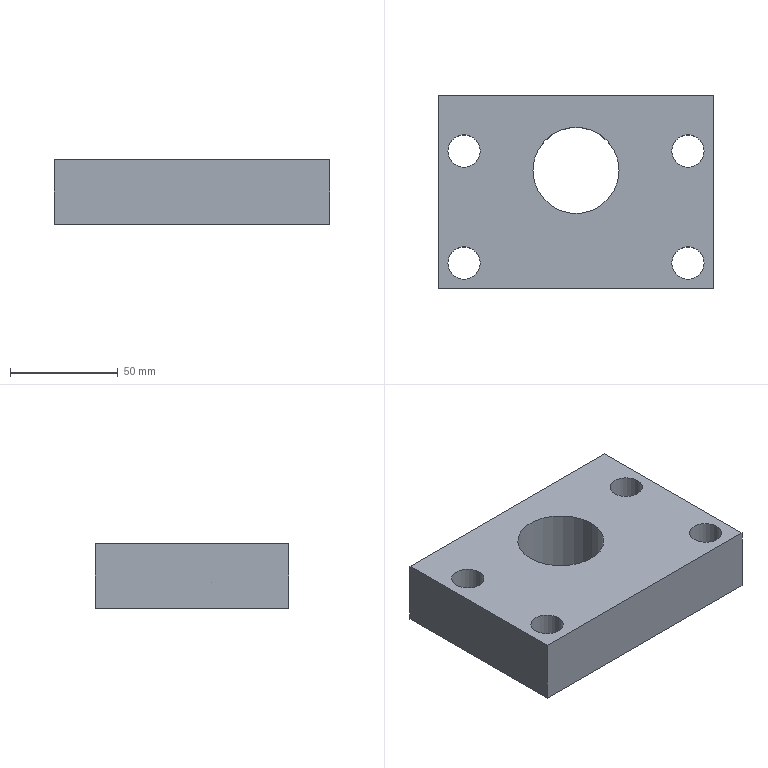Part | SolidWorks | features Extrusion 1, HoleWzd 1, ICE 1 | 1 solid | 16 faces | box 128 x 90 x 30 mm | volume 286695 mm3 | cylinder 10 | plane 6 | commonest cylinder face diameters 15 x8 40 x2
STEP:
#1=CARTESIAN_POINT('',(-59.5,19.,0.));
#2=VERTEX_POINT('',#1);
#3=CARTESIAN_POINT('',(-44.5,19.,0.));
#4=VERTEX_POINT('',#3);
#5=CARTESIAN_POINT('',(-52.,19.,0.));
#6=DIRECTION('',(0.,0.,1.));
#7=DIRECTION('',(1.,0.,0.));
#8=AXIS2_PLACEMENT_3D('',#5,#6,#7);
#9=CIRCLE('',#8,7.5);
#10=EDGE_CURVE('',#2,#4,#9,.T.);
#11=ORIENTED_EDGE('',*,*,#10,.F.);
#12=CARTESIAN_POINT('',(-59.5,19.,30.));
#13=VERTEX_POINT('',#12);
#14=CARTESIAN_POINT('',(-59.5,19.,30.));
#15=DIRECTION('',(0.,0.,1.));
#16=VECTOR('',#15,1000.);
#17=LINE('',#14,#16);
#18=EDGE_CURVE('',#2,#13,#17,.T.);
#19=ORIENTED_EDGE('',*,*,#18,.T.);
#20=CARTESIAN_POINT('',(-44.5,19.,30.));
#21=VERTEX_POINT('',#20);
#22=CARTESIAN_POINT('',(-52.,19.,30.));
#23=DIRECTION('',(0.,0.,1.));
#24=DIRECTION('',(1.,0.,0.));
#25=AXIS2_PLACEMENT_3D('',#22,#23,#24);
#26=CIRCLE('',#25,7.5);
#27=EDGE_CURVE('',#13,#21,#26,.T.);
#28=ORIENTED_EDGE('',*,*,#27,.T.);
#29=CARTESIAN_POINT('',(-44.5,19.,30.));
#30=DIRECTION('',(0.,0.,1.));
#31=VECTOR('',#30,1000.);
#32=LINE('',#29,#31);
#33=EDGE_CURVE('',#4,#21,#32,.T.);
#34=ORIENTED_EDGE('',*,*,#33,.F.);
#35=EDGE_LOOP('',(#11,#19,#28,#34));
#36=FACE_OUTER_BOUND('',#35,.T.);
#37=CARTESIAN_POINT('',(-52.,19.,30.));
#38=DIRECTION('',(0.,0.,1.));
#39=DIRECTION('',(1.,0.,0.));
#40=AXIS2_PLACEMENT_3D('',#37,#38,#39);
#41=CYLINDRICAL_SURFACE('',#40,7.5);
#42=ADVANCED_FACE('',(#36),#41,.F.);
#43=CARTESIAN_POINT('',(-59.5,-33.,0.));
#44=VERTEX_POINT('',#43);
#45=CARTESIAN_POINT('',(-44.5,-33.,0.));
#46=VERTEX_POINT('',#45);
#47=CARTESIAN_POINT('',(-52.,-33.,0.));
#48=DIRECTION('',(0.,0.,1.));
#49=DIRECTION('',(1.,0.,0.));
#50=AXIS2_PLACEMENT_3D('',#47,#48,#49);
#51=CIRCLE('',#50,7.5);
#52=EDGE_CURVE('',#44,#46,#51,.T.);
#53=ORIENTED_EDGE('',*,*,#52,.F.);
#54=CARTESIAN_POINT('',(-59.5,-33.,30.));
#55=VERTEX_POINT('',#54);
#56=CARTESIAN_POINT('',(-59.5,-33.,30.));
#57=DIRECTION('',(0.,0.,1.));
#58=VECTOR('',#57,1000.);
#59=LINE('',#56,#58);
#60=EDGE_CURVE('',#44,#55,#59,.T.);
#61=ORIENTED_EDGE('',*,*,#60,.T.);
#62=CARTESIAN_POINT('',(-44.5,-33.,30.));
#63=VERTEX_POINT('',#62);
#64=CARTESIAN_POINT('',(-52.,-33.,30.));
#65=DIRECTION('',(0.,0.,1.));
#66=DIRECTION('',(1.,0.,0.));
#67=AXIS2_PLACEMENT_3D('',#64,#65,#66);
#68=CIRCLE('',#67,7.5);
#69=EDGE_CURVE('',#55,#63,#68,.T.);
#70=ORIENTED_EDGE('',*,*,#69,.T.);
#71=CARTESIAN_POINT('',(-44.5,-33.,30.));
#72=DIRECTION('',(0.,0.,1.));
#73=VECTOR('',#72,1000.);
#74=LINE('',#71,#73);
#75=EDGE_CURVE('',#46,#63,#74,.T.);
#76=ORIENTED_EDGE('',*,*,#75,.F.);
#77=EDGE_LOOP('',(#53,#61,#70,#76));
#78=FACE_OUTER_BOUND('',#77,.T.);
#79=CARTESIAN_POINT('',(-52.,-33.,30.));
#80=DIRECTION('',(0.,0.,1.));
#81=DIRECTION('',(1.,0.,0.));
#82=AXIS2_PLACEMENT_3D('',#79,#80,#81);
#83=CYLINDRICAL_SURFACE('',#82,7.5);
#84=ADVANCED_FACE('',(#78),#83,.F.);
#85=CARTESIAN_POINT('',(44.5,-33.,0.));
#86=VERTEX_POINT('',#85);
#87=CARTESIAN_POINT('',(59.5,-33.,0.));
#88=VERTEX_POINT('',#87);
#89=CARTESIAN_POINT('',(52.,-33.,0.));
#90=DIRECTION('',(0.,0.,1.));
#91=DIRECTION('',(1.,0.,0.));
#92=AXIS2_PLACEMENT_3D('',#89,#90,#91);
#93=CIRCLE('',#92,7.5);
#94=EDGE_CURVE('',#86,#88,#93,.T.);
#95=ORIENTED_EDGE('',*,*,#94,.F.);
#96=CARTESIAN_POINT('',(44.5,-33.,30.));
#97=VERTEX_POINT('',#96);
#98=CARTESIAN_POINT('',(44.5,-33.,30.));
#99=DIRECTION('',(0.,0.,1.));
#100=VECTOR('',#99,1000.);
#101=LINE('',#98,#100);
#102=EDGE_CURVE('',#86,#97,#101,.T.);
#103=ORIENTED_EDGE('',*,*,#102,.T.);
#104=CARTESIAN_POINT('',(59.5,-33.,30.));
#105=VERTEX_POINT('',#104);
#106=CARTESIAN_POINT('',(52.,-33.,30.));
#107=DIRECTION('',(0.,0.,1.));
#108=DIRECTION('',(1.,0.,0.));
#109=AXIS2_PLACEMENT_3D('',#106,#107,#108);
#110=CIRCLE('',#109,7.5);
#111=EDGE_CURVE('',#97,#105,#110,.T.);
#112=ORIENTED_EDGE('',*,*,#111,.T.);
#113=CARTESIAN_POINT('',(59.5,-33.,30.));
#114=DIRECTION('',(0.,0.,1.));
#115=VECTOR('',#114,1000.);
#116=LINE('',#113,#115);
#117=EDGE_CURVE('',#88,#105,#116,.T.);
#118=ORIENTED_EDGE('',*,*,#117,.F.);
#119=EDGE_LOOP('',(#95,#103,#112,#118));
#120=FACE_OUTER_BOUND('',#119,.T.);
#121=CARTESIAN_POINT('',(52.,-33.,30.));
#122=DIRECTION('',(0.,0.,1.));
#123=DIRECTION('',(1.,0.,0.));
#124=AXIS2_PLACEMENT_3D('',#121,#122,#123);
#125=CYLINDRICAL_SURFACE('',#124,7.5);
#126=ADVANCED_FACE('',(#120),#125,.F.);
#127=CARTESIAN_POINT('',(44.5,19.,0.));
#128=VERTEX_POINT('',#127);
#129=CARTESIAN_POINT('',(59.5,19.,0.));
#130=VERTEX_POINT('',#129);
#131=CARTESIAN_POINT('',(52.,19.,0.));
#132=DIRECTION('',(0.,0.,1.));
#133=DIRECTION('',(1.,0.,0.));
#134=AXIS2_PLACEMENT_3D('',#131,#132,#133);
#135=CIRCLE('',#134,7.5);
#136=EDGE_CURVE('',#128,#130,#135,.T.);
#137=ORIENTED_EDGE('',*,*,#136,.F.);
#138=CARTESIAN_POINT('',(44.5,19.,30.));
#139=VERTEX_POINT('',#138);
#140=CARTESIAN_POINT('',(44.5,19.,30.));
#141=DIRECTION('',(0.,0.,1.));
#142=VECTOR('',#141,1000.);
#143=LINE('',#140,#142);
#144=EDGE_CURVE('',#128,#139,#143,.T.);
#145=ORIENTED_EDGE('',*,*,#144,.T.);
#146=CARTESIAN_POINT('',(59.5,19.,30.));
#147=VERTEX_POINT('',#146);
#148=CARTESIAN_POINT('',(52.,19.,30.));
#149=DIRECTION('',(0.,0.,1.));
#150=DIRECTION('',(1.,0.,0.));
#151=AXIS2_PLACEMENT_3D('',#148,#149,#150);
#152=CIRCLE('',#151,7.5);
#153=EDGE_CURVE('',#139,#147,#152,.T.);
#154=ORIENTED_EDGE('',*,*,#153,.T.);
#155=CARTESIAN_POINT('',(59.5,19.,30.));
#156=DIRECTION('',(0.,0.,1.));
#157=VECTOR('',#156,1000.);
#158=LINE('',#155,#157);
#159=EDGE_CURVE('',#130,#147,#158,.T.);
#160=ORIENTED_EDGE('',*,*,#159,.F.);
#161=EDGE_LOOP('',(#137,#145,#154,#160));
#162=FACE_OUTER_BOUND('',#161,.T.);
#163=CARTESIAN_POINT('',(52.,19.,30.));
#164=DIRECTION('',(0.,0.,1.));
#165=DIRECTION('',(1.,0.,0.));
#166=AXIS2_PLACEMENT_3D('',#163,#164,#165);
#167=CYLINDRICAL_SURFACE('',#166,7.5);
#168=ADVANCED_FACE('',(#162),#167,.F.);
#169=CARTESIAN_POINT('',(-20.,10.,0.));
#170=VERTEX_POINT('',#169);
#171=CARTESIAN_POINT('',(20.,10.,0.));
#172=VERTEX_POINT('',#171);
#173=CARTESIAN_POINT('',(0.,10.,0.));
#174=DIRECTION('',(0.,0.,1.));
#175=DIRECTION('',(1.,0.,0.));
#176=AXIS2_PLACEMENT_3D('',#173,#174,#175);
#177=CIRCLE('',#176,20.);
#178=EDGE_CURVE('',#170,#172,#177,.T.);
#179=ORIENTED_EDGE('',*,*,#178,.F.);
#180=CARTESIAN_POINT('',(-20.,10.,30.));
#181=VERTEX_POINT('',#180);
#182=CARTESIAN_POINT('',(-20.,10.,0.));
#183=DIRECTION('',(0.,0.,1.));
#184=VECTOR('',#183,1000.);
#185=LINE('',#182,#184);
#186=EDGE_CURVE('',#170,#181,#185,.T.);
#187=ORIENTED_EDGE('',*,*,#186,.T.);
#188=CARTESIAN_POINT('',(20.,10.,30.));
#189=VERTEX_POINT('',#188);
#190=CARTESIAN_POINT('',(0.,10.,30.));
#191=DIRECTION('',(0.,0.,1.));
#192=DIRECTION('',(1.,0.,0.));
#193=AXIS2_PLACEMENT_3D('',#190,#191,#192);
#194=CIRCLE('',#193,20.);
#195=EDGE_CURVE('',#181,#189,#194,.T.);
#196=ORIENTED_EDGE('',*,*,#195,.T.);
#197=CARTESIAN_POINT('',(20.,10.,0.));
#198=DIRECTION('',(0.,0.,1.));
#199=VECTOR('',#198,1000.);
#200=LINE('',#197,#199);
#201=EDGE_CURVE('',#172,#189,#200,.T.);
#202=ORIENTED_EDGE('',*,*,#201,.F.);
#203=EDGE_LOOP('',(#179,#187,#196,#202));
#204=FACE_OUTER_BOUND('',#203,.T.);
#205=CARTESIAN_POINT('',(0.,10.,0.));
#206=DIRECTION('',(0.,0.,1.));
#207=DIRECTION('',(1.,0.,0.));
#208=AXIS2_PLACEMENT_3D('',#205,#206,#207);
#209=CYLINDRICAL_SURFACE('',#208,20.);
#210=ADVANCED_FACE('',(#204),#209,.F.);
#211=CARTESIAN_POINT('',(-64.,45.,0.));
#212=VERTEX_POINT('',#211);
#213=CARTESIAN_POINT('',(-64.,-45.,0.));
#214=VERTEX_POINT('',#213);
#215=CARTESIAN_POINT('',(-64.,-45.,0.));
#216=DIRECTION('',(0.,-1.,0.));
#217=VECTOR('',#216,1000.);
#218=LINE('',#215,#217);
#219=EDGE_CURVE('',#212,#214,#218,.T.);
#220=ORIENTED_EDGE('',*,*,#219,.T.);
#221=CARTESIAN_POINT('',(-64.,-45.,30.));
#222=VERTEX_POINT('',#221);
#223=CARTESIAN_POINT('',(-64.,-45.,30.));
#224=DIRECTION('',(0.,0.,-1.));
#225=VECTOR('',#224,1000.);
#226=LINE('',#223,#225);
#227=EDGE_CURVE('',#222,#214,#226,.T.);
#228=ORIENTED_EDGE('',*,*,#227,.F.);
#229=CARTESIAN_POINT('',(-64.,45.,30.));
#230=VERTEX_POINT('',#229);
#231=CARTESIAN_POINT('',(-64.,-45.,30.));
#232=DIRECTION('',(0.,-1.,0.));
#233=VECTOR('',#232,1000.);
#234=LINE('',#231,#233);
#235=EDGE_CURVE('',#230,#222,#234,.T.);
#236=ORIENTED_EDGE('',*,*,#235,.F.);
#237=CARTESIAN_POINT('',(-64.,45.,30.));
#238=DIRECTION('',(0.,0.,-1.));
#239=VECTOR('',#238,1000.);
#240=LINE('',#237,#239);
#241=EDGE_CURVE('',#230,#212,#240,.T.);
#242=ORIENTED_EDGE('',*,*,#241,.T.);
#243=EDGE_LOOP('',(#220,#228,#236,#242));
#244=FACE_OUTER_BOUND('',#243,.T.);
#245=CARTESIAN_POINT('',(-64.,-45.,30.));
#246=DIRECTION('',(1.,0.,0.));
#247=DIRECTION('',(0.,0.,-1.));
#248=AXIS2_PLACEMENT_3D('',#245,#246,#247);
#249=PLANE('',#248);
#250=ADVANCED_FACE('',(#244),#249,.F.);
#251=CARTESIAN_POINT('',(64.,-45.,0.));
#252=VERTEX_POINT('',#251);
#253=CARTESIAN_POINT('',(64.,-45.,0.));
#254=DIRECTION('',(1.,0.,0.));
#255=VECTOR('',#254,1000.);
#256=LINE('',#253,#255);
#257=EDGE_CURVE('',#214,#252,#256,.T.);
#258=ORIENTED_EDGE('',*,*,#257,.T.);
#259=CARTESIAN_POINT('',(64.,-45.,30.));
#260=VERTEX_POINT('',#259);
#261=CARTESIAN_POINT('',(64.,-45.,30.));
#262=DIRECTION('',(0.,0.,-1.));
#263=VECTOR('',#262,1000.);
#264=LINE('',#261,#263);
#265=EDGE_CURVE('',#260,#252,#264,.T.);
#266=ORIENTED_EDGE('',*,*,#265,.F.);
#267=CARTESIAN_POINT('',(64.,-45.,30.));
#268=DIRECTION('',(1.,0.,0.));
#269=VECTOR('',#268,1000.);
#270=LINE('',#267,#269);
#271=EDGE_CURVE('',#222,#260,#270,.T.);
#272=ORIENTED_EDGE('',*,*,#271,.F.);
#273=ORIENTED_EDGE('',*,*,#227,.T.);
#274=EDGE_LOOP('',(#258,#266,#272,#273));
#275=FACE_OUTER_BOUND('',#274,.T.);
#276=CARTESIAN_POINT('',(64.,-45.,30.));
#277=DIRECTION('',(0.,1.,0.));
#278=DIRECTION('',(-1.,0.,0.));
#279=AXIS2_PLACEMENT_3D('',#276,#277,#278);
#280=PLANE('',#279);
#281=ADVANCED_FACE('',(#275),#280,.F.);
#282=CARTESIAN_POINT('',(64.,45.,0.));
#283=VERTEX_POINT('',#282);
#284=CARTESIAN_POINT('',(64.,-45.,0.));
#285=DIRECTION('',(0.,1.,0.));
#286=VECTOR('',#285,1000.);
#287=LINE('',#284,#286);
#288=EDGE_CURVE('',#252,#283,#287,.T.);
#289=ORIENTED_EDGE('',*,*,#288,.T.);
#290=CARTESIAN_POINT('',(64.,45.,30.));
#291=VERTEX_POINT('',#290);
#292=CARTESIAN_POINT('',(64.,45.,30.));
#293=DIRECTION('',(0.,0.,-1.));
#294=VECTOR('',#293,1000.);
#295=LINE('',#292,#294);
#296=EDGE_CURVE('',#291,#283,#295,.T.);
#297=ORIENTED_EDGE('',*,*,#296,.F.);
#298=CARTESIAN_POINT('',(64.,-45.,30.));
#299=DIRECTION('',(0.,1.,0.));
#300=VECTOR('',#299,1000.);
#301=LINE('',#298,#300);
#302=EDGE_CURVE('',#260,#291,#301,.T.);
#303=ORIENTED_EDGE('',*,*,#302,.F.);
#304=ORIENTED_EDGE('',*,*,#265,.T.);
#305=EDGE_LOOP('',(#289,#297,#303,#304));
#306=FACE_OUTER_BOUND('',#305,.T.);
#307=CARTESIAN_POINT('',(64.,-45.,30.));
#308=DIRECTION('',(-1.,0.,0.));
#309=DIRECTION('',(0.,0.,1.));
#310=AXIS2_PLACEMENT_3D('',#307,#308,#309);
#311=PLANE('',#310);
#312=ADVANCED_FACE('',(#306),#311,.F.);
#313=CARTESIAN_POINT('',(64.,45.,0.));
#314=DIRECTION('',(-1.,0.,0.));
#315=VECTOR('',#314,1000.);
#316=LINE('',#313,#315);
#317=EDGE_CURVE('',#283,#212,#316,.T.);
#318=ORIENTED_EDGE('',*,*,#317,.T.);
#319=ORIENTED_EDGE('',*,*,#241,.F.);
#320=CARTESIAN_POINT('',(64.,45.,30.));
#321=DIRECTION('',(-1.,0.,0.));
#322=VECTOR('',#321,1000.);
#323=LINE('',#320,#322);
#324=EDGE_CURVE('',#291,#230,#323,.T.);
#325=ORIENTED_EDGE('',*,*,#324,.F.);
#326=ORIENTED_EDGE('',*,*,#296,.T.);
#327=EDGE_LOOP('',(#318,#319,#325,#326));
#328=FACE_OUTER_BOUND('',#327,.T.);
#329=CARTESIAN_POINT('',(64.,45.,30.));
#330=DIRECTION('',(0.,-1.,0.));
#331=DIRECTION('',(1.,0.,0.));
#332=AXIS2_PLACEMENT_3D('',#329,#330,#331);
#333=PLANE('',#332);
#334=ADVANCED_FACE('',(#328),#333,.F.);
#335=CARTESIAN_POINT('',(-52.,19.,30.));
#336=DIRECTION('',(0.,0.,1.));
#337=DIRECTION('',(1.,0.,0.));
#338=AXIS2_PLACEMENT_3D('',#335,#336,#337);
#339=CIRCLE('',#338,7.5);
#340=EDGE_CURVE('',#21,#13,#339,.T.);
#341=ORIENTED_EDGE('',*,*,#340,.F.);
#342=ORIENTED_EDGE('',*,*,#27,.F.);
#343=EDGE_LOOP('',(#341,#342));
#344=FACE_BOUND('',#343,.T.);
#345=CARTESIAN_POINT('',(-52.,-33.,30.));
#346=DIRECTION('',(0.,0.,1.));
#347=DIRECTION('',(1.,0.,0.));
#348=AXIS2_PLACEMENT_3D('',#345,#346,#347);
#349=CIRCLE('',#348,7.5);
#350=EDGE_CURVE('',#63,#55,#349,.T.);
#351=ORIENTED_EDGE('',*,*,#350,.F.);
#352=ORIENTED_EDGE('',*,*,#69,.F.);
#353=EDGE_LOOP('',(#351,#352));
#354=FACE_BOUND('',#353,.T.);
#355=CARTESIAN_POINT('',(52.,-33.,30.));
#356=DIRECTION('',(0.,0.,1.));
#357=DIRECTION('',(1.,0.,0.));
#358=AXIS2_PLACEMENT_3D('',#355,#356,#357);
#359=CIRCLE('',#358,7.5);
#360=EDGE_CURVE('',#105,#97,#359,.T.);
#361=ORIENTED_EDGE('',*,*,#360,.F.);
#362=ORIENTED_EDGE('',*,*,#111,.F.);
#363=EDGE_LOOP('',(#361,#362));
#364=FACE_BOUND('',#363,.T.);
#365=CARTESIAN_POINT('',(52.,19.,30.));
#366=DIRECTION('',(0.,0.,1.));
#367=DIRECTION('',(1.,0.,0.));
#368=AXIS2_PLACEMENT_3D('',#365,#366,#367);
#369=CIRCLE('',#368,7.5);
#370=EDGE_CURVE('',#147,#139,#369,.T.);
#371=ORIENTED_EDGE('',*,*,#370,.F.);
#372=ORIENTED_EDGE('',*,*,#153,.F.);
#373=EDGE_LOOP('',(#371,#372));
#374=FACE_BOUND('',#373,.T.);
#375=CARTESIAN_POINT('',(0.,10.,30.));
#376=DIRECTION('',(0.,0.,1.));
#377=DIRECTION('',(1.,0.,0.));
#378=AXIS2_PLACEMENT_3D('',#375,#376,#377);
#379=CIRCLE('',#378,20.);
#380=EDGE_CURVE('',#189,#181,#379,.T.);
#381=ORIENTED_EDGE('',*,*,#380,.F.);
#382=ORIENTED_EDGE('',*,*,#195,.F.);
#383=EDGE_LOOP('',(#381,#382));
#384=FACE_BOUND('',#383,.T.);
#385=ORIENTED_EDGE('',*,*,#235,.T.);
#386=ORIENTED_EDGE('',*,*,#271,.T.);
#387=ORIENTED_EDGE('',*,*,#302,.T.);
#388=ORIENTED_EDGE('',*,*,#324,.T.);
#389=EDGE_LOOP('',(#385,#386,#387,#388));
#390=FACE_OUTER_BOUND('',#389,.T.);
#391=CARTESIAN_POINT('',(0.,0.,30.));
#392=DIRECTION('',(0.,0.,1.));
#393=DIRECTION('',(1.,0.,0.));
#394=AXIS2_PLACEMENT_3D('',#391,#392,#393);
#395=PLANE('',#394);
#396=ADVANCED_FACE('',(#344,#354,#364,#374,#384,#390),#395,.T.);
#397=CARTESIAN_POINT('',(-52.,19.,0.));
#398=DIRECTION('',(0.,0.,1.));
#399=DIRECTION('',(1.,0.,0.));
#400=AXIS2_PLACEMENT_3D('',#397,#398,#399);
#401=CIRCLE('',#400,7.5);
#402=EDGE_CURVE('',#4,#2,#401,.T.);
#403=ORIENTED_EDGE('',*,*,#402,.T.);
#404=ORIENTED_EDGE('',*,*,#10,.T.);
#405=EDGE_LOOP('',(#403,#404));
#406=FACE_BOUND('',#405,.T.);
#407=CARTESIAN_POINT('',(-52.,-33.,0.));
#408=DIRECTION('',(0.,0.,1.));
#409=DIRECTION('',(1.,0.,0.));
#410=AXIS2_PLACEMENT_3D('',#407,#408,#409);
#411=CIRCLE('',#410,7.5);
#412=EDGE_CURVE('',#46,#44,#411,.T.);
#413=ORIENTED_EDGE('',*,*,#412,.T.);
#414=ORIENTED_EDGE('',*,*,#52,.T.);
#415=EDGE_LOOP('',(#413,#414));
#416=FACE_BOUND('',#415,.T.);
#417=CARTESIAN_POINT('',(52.,-33.,0.));
#418=DIRECTION('',(0.,0.,1.));
#419=DIRECTION('',(1.,0.,0.));
#420=AXIS2_PLACEMENT_3D('',#417,#418,#419);
#421=CIRCLE('',#420,7.5);
#422=EDGE_CURVE('',#88,#86,#421,.T.);
#423=ORIENTED_EDGE('',*,*,#422,.T.);
#424=ORIENTED_EDGE('',*,*,#94,.T.);
#425=EDGE_LOOP('',(#423,#424));
#426=FACE_BOUND('',#425,.T.);
#427=CARTESIAN_POINT('',(52.,19.,0.));
#428=DIRECTION('',(0.,0.,1.));
#429=DIRECTION('',(1.,0.,0.));
#430=AXIS2_PLACEMENT_3D('',#427,#428,#429);
#431=CIRCLE('',#430,7.5);
#432=EDGE_CURVE('',#130,#128,#431,.T.);
#433=ORIENTED_EDGE('',*,*,#432,.T.);
#434=ORIENTED_EDGE('',*,*,#136,.T.);
#435=EDGE_LOOP('',(#433,#434));
#436=FACE_BOUND('',#435,.T.);
#437=CARTESIAN_POINT('',(0.,10.,0.));
#438=DIRECTION('',(0.,0.,1.));
#439=DIRECTION('',(1.,0.,0.));
#440=AXIS2_PLACEMENT_3D('',#437,#438,#439);
#441=CIRCLE('',#440,20.);
#442=EDGE_CURVE('',#172,#170,#441,.T.);
#443=ORIENTED_EDGE('',*,*,#442,.T.);
#444=ORIENTED_EDGE('',*,*,#178,.T.);
#445=EDGE_LOOP('',(#443,#444));
#446=FACE_BOUND('',#445,.T.);
#447=ORIENTED_EDGE('',*,*,#219,.F.);
#448=ORIENTED_EDGE('',*,*,#317,.F.);
#449=ORIENTED_EDGE('',*,*,#288,.F.);
#450=ORIENTED_EDGE('',*,*,#257,.F.);
#451=EDGE_LOOP('',(#447,#448,#449,#450));
#452=FACE_OUTER_BOUND('',#451,.T.);
#453=CARTESIAN_POINT('',(0.,0.,0.));
#454=DIRECTION('',(0.,0.,1.));
#455=DIRECTION('',(1.,0.,0.));
#456=AXIS2_PLACEMENT_3D('',#453,#454,#455);
#457=PLANE('',#456);
#458=ADVANCED_FACE('',(#406,#416,#426,#436,#446,#452),#457,.F.);
#459=ORIENTED_EDGE('',*,*,#186,.F.);
#460=ORIENTED_EDGE('',*,*,#442,.F.);
#461=ORIENTED_EDGE('',*,*,#201,.T.);
#462=ORIENTED_EDGE('',*,*,#380,.T.);
#463=EDGE_LOOP('',(#459,#460,#461,#462));
#464=FACE_OUTER_BOUND('',#463,.T.);
#465=CARTESIAN_POINT('',(0.,10.,0.));
#466=DIRECTION('',(0.,0.,1.));
#467=DIRECTION('',(1.,0.,0.));
#468=AXIS2_PLACEMENT_3D('',#465,#466,#467);
#469=CYLINDRICAL_SURFACE('',#468,20.);
#470=ADVANCED_FACE('',(#464),#469,.F.);
#471=ORIENTED_EDGE('',*,*,#144,.F.);
#472=ORIENTED_EDGE('',*,*,#432,.F.);
#473=ORIENTED_EDGE('',*,*,#159,.T.);
#474=ORIENTED_EDGE('',*,*,#370,.T.);
#475=EDGE_LOOP('',(#471,#472,#473,#474));
#476=FACE_OUTER_BOUND('',#475,.T.);
#477=CARTESIAN_POINT('',(52.,19.,30.));
#478=DIRECTION('',(0.,0.,1.));
#479=DIRECTION('',(1.,0.,0.));
#480=AXIS2_PLACEMENT_3D('',#477,#478,#479);
#481=CYLINDRICAL_SURFACE('',#480,7.5);
#482=ADVANCED_FACE('',(#476),#481,.F.);
#483=ORIENTED_EDGE('',*,*,#102,.F.);
#484=ORIENTED_EDGE('',*,*,#422,.F.);
#485=ORIENTED_EDGE('',*,*,#117,.T.);
#486=ORIENTED_EDGE('',*,*,#360,.T.);
#487=EDGE_LOOP('',(#483,#484,#485,#486));
#488=FACE_OUTER_BOUND('',#487,.T.);
#489=CARTESIAN_POINT('',(52.,-33.,30.));
#490=DIRECTION('',(0.,0.,1.));
#491=DIRECTION('',(1.,0.,0.));
#492=AXIS2_PLACEMENT_3D('',#489,#490,#491);
#493=CYLINDRICAL_SURFACE('',#492,7.5);
#494=ADVANCED_FACE('',(#488),#493,.F.);
#495=ORIENTED_EDGE('',*,*,#60,.F.);
#496=ORIENTED_EDGE('',*,*,#412,.F.);
#497=ORIENTED_EDGE('',*,*,#75,.T.);
#498=ORIENTED_EDGE('',*,*,#350,.T.);
#499=EDGE_LOOP('',(#495,#496,#497,#498));
#500=FACE_OUTER_BOUND('',#499,.T.);
#501=CARTESIAN_POINT('',(-52.,-33.,30.));
#502=DIRECTION('',(0.,0.,1.));
#503=DIRECTION('',(1.,0.,0.));
#504=AXIS2_PLACEMENT_3D('',#501,#502,#503);
#505=CYLINDRICAL_SURFACE('',#504,7.5);
#506=ADVANCED_FACE('',(#500),#505,.F.);
#507=ORIENTED_EDGE('',*,*,#18,.F.);
#508=ORIENTED_EDGE('',*,*,#402,.F.);
#509=ORIENTED_EDGE('',*,*,#33,.T.);
#510=ORIENTED_EDGE('',*,*,#340,.T.);
#511=EDGE_LOOP('',(#507,#508,#509,#510));
#512=FACE_OUTER_BOUND('',#511,.T.);
#513=CARTESIAN_POINT('',(-52.,19.,30.));
#514=DIRECTION('',(0.,0.,1.));
#515=DIRECTION('',(1.,0.,0.));
#516=AXIS2_PLACEMENT_3D('',#513,#514,#515);
#517=CYLINDRICAL_SURFACE('',#516,7.5);
#518=ADVANCED_FACE('',(#512),#517,.F.);
#519=CLOSED_SHELL('',(#42,#84,#126,#168,#210,#250,#281,#312,#334,#396,#458,#470,#482,#494,#506,#518));
#520=MANIFOLD_SOLID_BREP('',#519);
#521=CARTESIAN_POINT('',(0.,0.,0.));
#522=DIRECTION('',(0.,0.,1.));
#523=DIRECTION('',(1.,0.,0.));
#524=AXIS2_PLACEMENT_3D('',#521,#522,#523);
#525=(LENGTH_UNIT()NAMED_UNIT(*)SI_UNIT(.MILLI.,.METRE.));
#526=UNCERTAINTY_MEASURE_WITH_UNIT(LENGTH_MEASURE(0.00001),#525,'','');
#527=(NAMED_UNIT(*)PLANE_ANGLE_UNIT()SI_UNIT($,.RADIAN.));
#528=(NAMED_UNIT(*)SI_UNIT($,.STERADIAN.)SOLID_ANGLE_UNIT());
#529=(GEOMETRIC_REPRESENTATION_CONTEXT(3)GLOBAL_UNCERTAINTY_ASSIGNED_CONTEXT((#526))GLOBAL_UNIT_ASSIGNED_CONTEXT((#525,#527,#528))REPRESENTATION_CONTEXT('',''));
#530=ADVANCED_BREP_SHAPE_REPRESENTATION('',(#520,#524),#529);